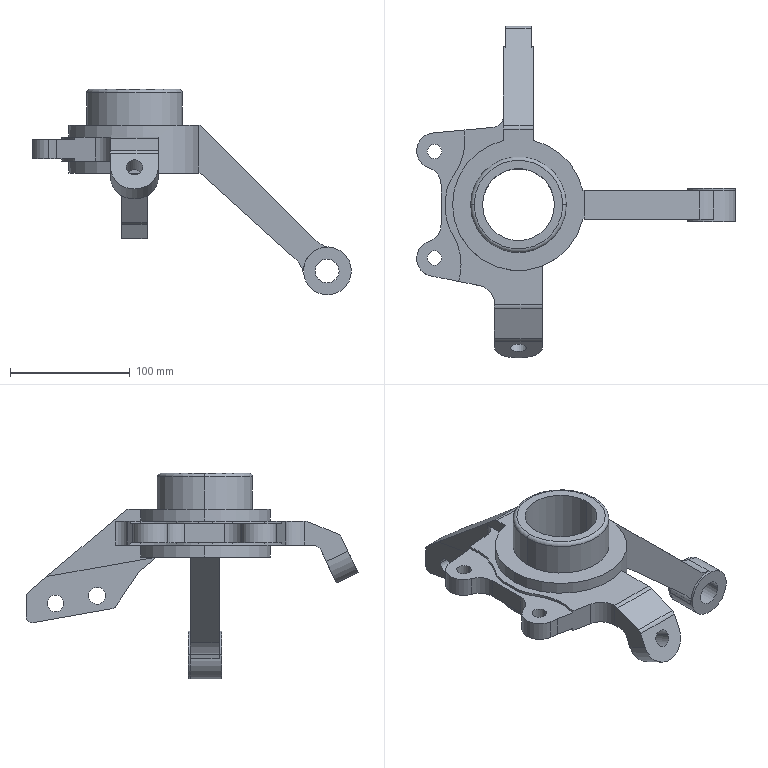Part | SolidWorks | features MBimport 1 | 2 solids | 95 faces | box 266.066 x 277.183 x 171.657 mm | volume 646593 mm3 | cylinder 58 | plane 35 | torus 2 | commonest cylinder face diameters 100 x8 40 x7 14 x6 60 x6 10 x5 12 x4